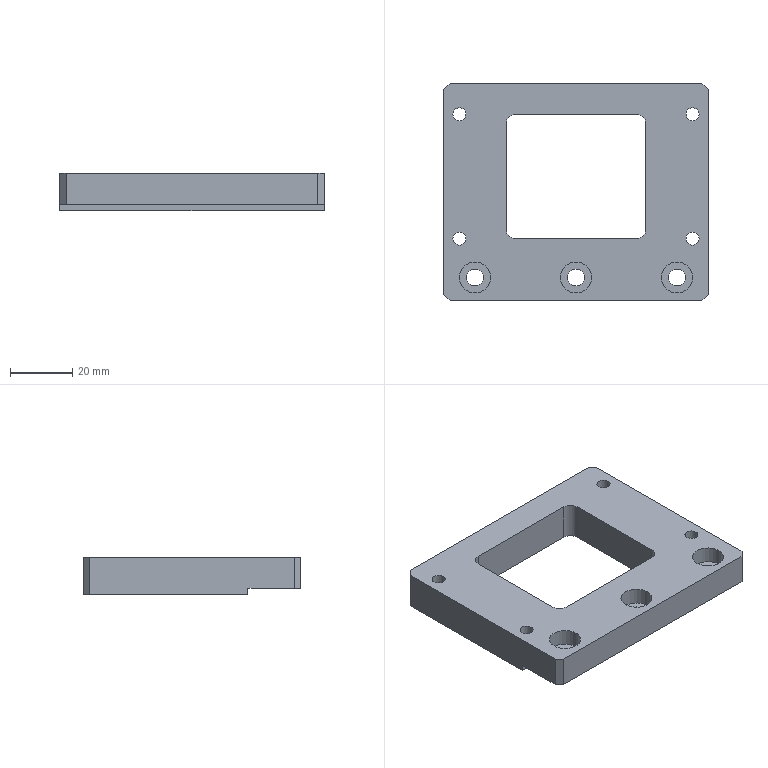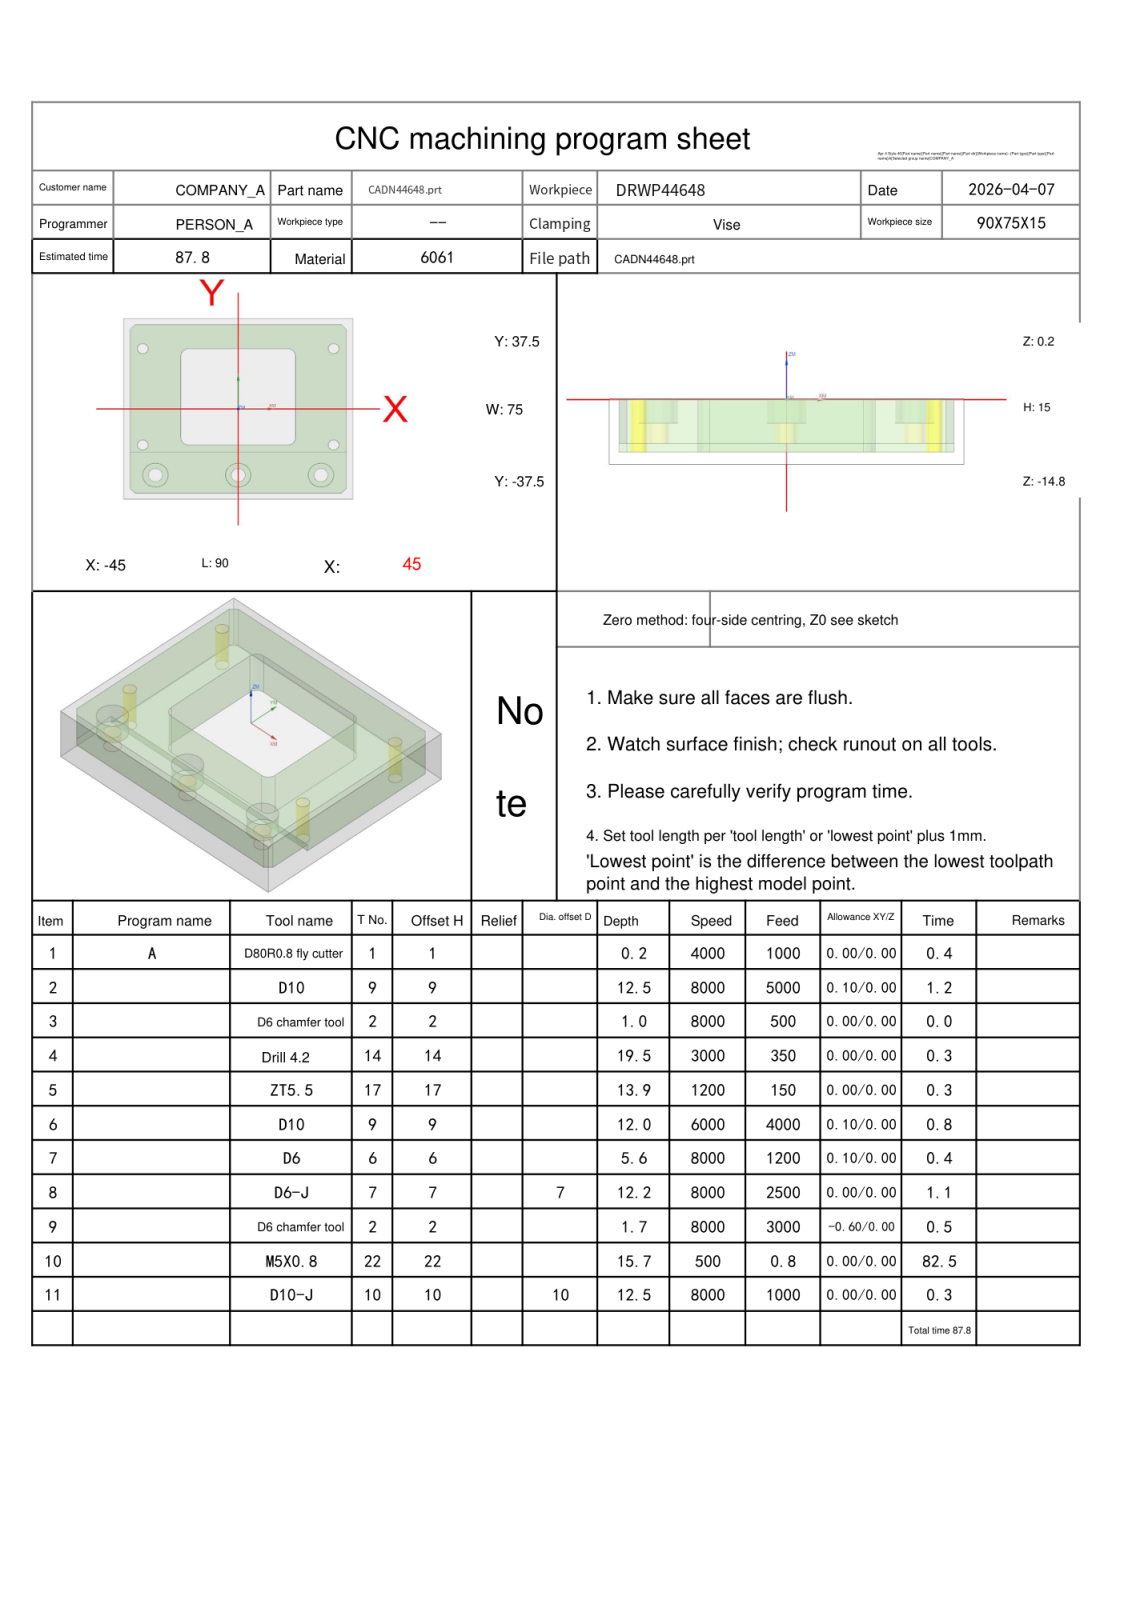NC program | NX | posted by the shop | part box 85 x 70 x 12 mm
Lines 1 to 579 of 5800:
%
O0001
(Machine time: 167.60 MIN)
(===Total Tool:9===)
(T1=D80R0.8 fly cutter D=80.  R=0.8  D-  H01 Z=0.    )
(T9=D10     D=10.  R=0.   D-  H09 Z=-12.3 )
(T2=D6 chamfer tool   D=6.   R=0.   D-  H02 Z=-1.5  )
(T14=drill 4.2  D=4.2  DR_a=118 D-  H14 Z=-19.26)
(T17=ZT5.5  D=5.5  DR_a=118 D-  H17 Z=-13.65)
(T6=D6      D=6.   R=0.   D-  H06 Z=-5.4  )
(T7=D6-J    D=6.   R=0.   D7  H07 Z=-12.  )
(T22=M5X0.8 D=4.2  DR_a=180 D-  H22 Z=-15.5 )
(T10=D10-J  D=10.  R=0.   D10 H10 Z=-12.3 )
G80 G90 G17 G49 G40
G91 G28 Z0
M01
N1 T01 M06
(D80R0.8 fly cutter  D=80. R=0.8 H=01 ce=0.00 di=0.00)
G00 G90 G54 X-87.5 Y25. M03 S4000
G43 H01 Z20.
M08
Z2.
G01 Z0.0 F1000.
X-82.5
X82.5
Y-25.
X-82.5
X-87.5
Z2.
G00 Z20.
G91 G28 Z0.0
M05
M09
G91 G28 Z0.0
M01
N2 T09 M06
(D10  D=10. R=0. H=09 ce=0.10 di=0.00)
G00 G90 G54 X0.0 Y40.1 M03 S8000
G43 H09 Z20.
M08
Z.5
G01 X40.5 Z.404 F5000.
G02 X44.106 Y38.606 Z.394 I0.0 J-5.1
G01 X46.106 Y36.606 Z.388
G02 X47.6 Y33. Z.378 I-3.606 J-3.606
G01 Y-33. Z.222
G02 X46.106 Y-36.606 Z.212 I-5.1 J0.0
G01 X44.106 Y-38.606 Z.206
G02 X40.5 Y-40.1 Z.196 I-3.606 J3.606
G01 X-40.5 Z.004
G02 X-44.106 Y-38.606 Z-.006 I0.0 J5.1
G01 X-46.106 Y-36.606 Z-.012
G02 X-47.6 Y-33. Z-.022 I3.606 J3.606
G01 Y33. Z-.178
G02 X-46.106 Y36.606 Z-.188 I5.1 J0.0
G01 X-44.106 Y38.606 Z-.194
G02 X-40.5 Y40.1 Z-.204 I3.606 J-3.606
G01 X40.5 Z-.396
G02 X44.106 Y38.606 Z-.406 I0.0 J-5.1
G01 X46.106 Y36.606 Z-.412
G02 X47.6 Y33. Z-.422 I-3.606 J-3.606
G01 Y-33. Z-.578
G02 X46.106 Y-36.606 Z-.588 I-5.1 J0.0
G01 X44.106 Y-38.606 Z-.594
G02 X40.5 Y-40.1 Z-.604 I-3.606 J3.606
G01 X-40.5 Z-.796
G02 X-44.106 Y-38.606 Z-.806 I0.0 J5.1
G01 X-46.106 Y-36.606 Z-.812
G02 X-47.6 Y-33. Z-.822 I3.606 J3.606
G01 Y33. Z-.978
G02 X-46.106 Y36.606 Z-.988 I5.1 J0.0
G01 X-44.106 Y38.606 Z-.994
G02 X-40.5 Y40.1 Z-1.004 I3.606 J-3.606
G01 X40.5 Z-1.196
G02 X44.106 Y38.606 Z-1.206 I0.0 J-5.1
G01 X46.106 Y36.606 Z-1.212
G02 X47.6 Y33. Z-1.222 I-3.606 J-3.606
G01 Y-33. Z-1.378
G02 X46.106 Y-36.606 Z-1.388 I-5.1 J0.0
G01 X44.106 Y-38.606 Z-1.394
G02 X40.5 Y-40.1 Z-1.404 I-3.606 J3.606
G01 X-40.5 Z-1.596
G02 X-44.106 Y-38.606 Z-1.606 I0.0 J5.1
G01 X-46.106 Y-36.606 Z-1.612
G02 X-47.6 Y-33. Z-1.622 I3.606 J3.606
G01 Y33. Z-1.778
G02 X-46.106 Y36.606 Z-1.788 I5.1 J0.0
G01 X-44.106 Y38.606 Z-1.794
G02 X-40.5 Y40.1 Z-1.804 I3.606 J-3.606
G01 X40.5 Z-1.996
G02 X44.106 Y38.606 Z-2.006 I0.0 J-5.1
G01 X46.106 Y36.606 Z-2.012
G02 X47.6 Y33. Z-2.022 I-3.606 J-3.606
G01 Y-33. Z-2.178
G02 X46.106 Y-36.606 Z-2.188 I-5.1 J0.0
G01 X44.106 Y-38.606 Z-2.194
G02 X40.5 Y-40.1 Z-2.204 I-3.606 J3.606
G01 X-40.5 Z-2.396
G02 X-44.106 Y-38.606 Z-2.406 I0.0 J5.1
G01 X-46.106 Y-36.606 Z-2.412
G02 X-47.6 Y-33. Z-2.422 I3.606 J3.606
G01 Y33. Z-2.578
G02 X-46.106 Y36.606 Z-2.588 I5.1 J0.0
G01 X-44.106 Y38.606 Z-2.594
G02 X-40.5 Y40.1 Z-2.604 I3.606 J-3.606
G01 X40.5 Z-2.796
G02 X44.106 Y38.606 Z-2.806 I0.0 J-5.1
G01 X46.106 Y36.606 Z-2.812
G02 X47.6 Y33. Z-2.822 I-3.606 J-3.606
G01 Y-33. Z-2.978
G02 X46.106 Y-36.606 Z-2.988 I-5.1 J0.0
G01 X44.106 Y-38.606 Z-2.994
G02 X40.5 Y-40.1 Z-3.004 I-3.606 J3.606
G01 X-40.5 Z-3.196
G02 X-44.106 Y-38.606 Z-3.206 I0.0 J5.1
G01 X-46.106 Y-36.606 Z-3.212
G02 X-47.6 Y-33. Z-3.222 I3.606 J3.606
G01 Y33. Z-3.378
G02 X-46.106 Y36.606 Z-3.388 I5.1 J0.0
G01 X-44.106 Y38.606 Z-3.394
G02 X-40.5 Y40.1 Z-3.404 I3.606 J-3.606
G01 X40.5 Z-3.596
G02 X44.106 Y38.606 Z-3.606 I0.0 J-5.1
G01 X46.106 Y36.606 Z-3.612
G02 X47.6 Y33. Z-3.622 I-3.606 J-3.606
G01 Y-33. Z-3.778
G02 X46.106 Y-36.606 Z-3.788 I-5.1 J0.0
G01 X44.106 Y-38.606 Z-3.794
G02 X40.5 Y-40.1 Z-3.804 I-3.606 J3.606
G01 X-40.5 Z-3.996
G02 X-44.106 Y-38.606 Z-4.006 I0.0 J5.1
G01 X-46.106 Y-36.606 Z-4.012
G02 X-47.6 Y-33. Z-4.022 I3.606 J3.606
G01 Y33. Z-4.178
G02 X-46.106 Y36.606 Z-4.188 I5.1 J0.0
G01 X-44.106 Y38.606 Z-4.194
G02 X-40.5 Y40.1 Z-4.204 I3.606 J-3.606
G01 X40.5 Z-4.396
G02 X44.106 Y38.606 Z-4.406 I0.0 J-5.1
G01 X46.106 Y36.606 Z-4.412
G02 X47.6 Y33. Z-4.422 I-3.606 J-3.606
G01 Y-33. Z-4.578
G02 X46.106 Y-36.606 Z-4.588 I-5.1 J0.0
G01 X44.106 Y-38.606 Z-4.594
G02 X40.5 Y-40.1 Z-4.604 I-3.606 J3.606
G01 X-40.5 Z-4.796
G02 X-44.106 Y-38.606 Z-4.806 I0.0 J5.1
G01 X-46.106 Y-36.606 Z-4.812
G02 X-47.6 Y-33. Z-4.822 I3.606 J3.606
G01 Y33. Z-4.978
G02 X-46.106 Y36.606 Z-4.988 I5.1 J0.0
G01 X-44.106 Y38.606 Z-4.994
G02 X-40.5 Y40.1 Z-5.004 I3.606 J-3.606
G01 X40.5 Z-5.196
G02 X44.106 Y38.606 Z-5.206 I0.0 J-5.1
G01 X46.106 Y36.606 Z-5.212
G02 X47.6 Y33. Z-5.222 I-3.606 J-3.606
G01 Y-33. Z-5.378
G02 X46.106 Y-36.606 Z-5.388 I-5.1 J0.0
G01 X44.106 Y-38.606 Z-5.394
G02 X40.5 Y-40.1 Z-5.404 I-3.606 J3.606
G01 X-40.5 Z-5.596
G02 X-44.106 Y-38.606 Z-5.606 I0.0 J5.1
G01 X-46.106 Y-36.606 Z-5.612
G02 X-47.6 Y-33. Z-5.622 I3.606 J3.606
G01 Y33. Z-5.778
G02 X-46.106 Y36.606 Z-5.788 I5.1 J0.0
G01 X-44.106 Y38.606 Z-5.794
G02 X-40.5 Y40.1 Z-5.804 I3.606 J-3.606
G01 X40.5 Z-5.996
G02 X44.106 Y38.606 Z-6.006 I0.0 J-5.1
G01 X46.106 Y36.606 Z-6.012
G02 X47.6 Y33. Z-6.022 I-3.606 J-3.606
G01 Y-33. Z-6.178
G02 X46.106 Y-36.606 Z-6.188 I-5.1 J0.0
G01 X44.106 Y-38.606 Z-6.194
G02 X40.5 Y-40.1 Z-6.204 I-3.606 J3.606
G01 X-40.5 Z-6.396
G02 X-44.106 Y-38.606 Z-6.406 I0.0 J5.1
G01 X-46.106 Y-36.606 Z-6.412
G02 X-47.6 Y-33. Z-6.422 I3.606 J3.606
G01 Y33. Z-6.578
G02 X-46.106 Y36.606 Z-6.588 I5.1 J0.0
G01 X-44.106 Y38.606 Z-6.594
G02 X-40.5 Y40.1 Z-6.604 I3.606 J-3.606
G01 X40.5 Z-6.796
G02 X44.106 Y38.606 Z-6.806 I0.0 J-5.1
G01 X46.106 Y36.606 Z-6.812
G02 X47.6 Y33. Z-6.822 I-3.606 J-3.606
G01 Y-33. Z-6.978
G02 X46.106 Y-36.606 Z-6.988 I-5.1 J0.0
G01 X44.106 Y-38.606 Z-6.994
G02 X40.5 Y-40.1 Z-7.004 I-3.606 J3.606
G01 X-40.5 Z-7.196
G02 X-44.106 Y-38.606 Z-7.206 I0.0 J5.1
G01 X-46.106 Y-36.606 Z-7.212
G02 X-47.6 Y-33. Z-7.222 I3.606 J3.606
G01 Y33. Z-7.378
G02 X-46.106 Y36.606 Z-7.388 I5.1 J0.0
G01 X-44.106 Y38.606 Z-7.394
G02 X-40.5 Y40.1 Z-7.404 I3.606 J-3.606
G01 X40.5 Z-7.596
G02 X44.106 Y38.606 Z-7.606 I0.0 J-5.1
G01 X46.106 Y36.606 Z-7.612
G02 X47.6 Y33. Z-7.622 I-3.606 J-3.606
G01 Y-33. Z-7.778
G02 X46.106 Y-36.606 Z-7.788 I-5.1 J0.0
G01 X44.106 Y-38.606 Z-7.794
G02 X40.5 Y-40.1 Z-7.804 I-3.606 J3.606
G01 X-40.5 Z-7.996
G02 X-44.106 Y-38.606 Z-8.006 I0.0 J5.1
G01 X-46.106 Y-36.606 Z-8.012
G02 X-47.6 Y-33. Z-8.022 I3.606 J3.606
G01 Y33. Z-8.178
G02 X-46.106 Y36.606 Z-8.188 I5.1 J0.0
G01 X-44.106 Y38.606 Z-8.194
G02 X-40.5 Y40.1 Z-8.204 I3.606 J-3.606
G01 X40.5 Z-8.396
G02 X44.106 Y38.606 Z-8.406 I0.0 J-5.1
G01 X46.106 Y36.606 Z-8.412
G02 X47.6 Y33. Z-8.422 I-3.606 J-3.606
G01 Y-33. Z-8.578
G02 X46.106 Y-36.606 Z-8.588 I-5.1 J0.0
G01 X44.106 Y-38.606 Z-8.594
G02 X40.5 Y-40.1 Z-8.604 I-3.606 J3.606
G01 X-40.5 Z-8.796
G02 X-44.106 Y-38.606 Z-8.806 I0.0 J5.1
G01 X-46.106 Y-36.606 Z-8.812
G02 X-47.6 Y-33. Z-8.822 I3.606 J3.606
G01 Y33. Z-8.978
G02 X-46.106 Y36.606 Z-8.988 I5.1 J0.0
G01 X-44.106 Y38.606 Z-8.994
G02 X-40.5 Y40.1 Z-9.004 I3.606 J-3.606
G01 X40.5 Z-9.196
G02 X44.106 Y38.606 Z-9.206 I0.0 J-5.1
G01 X46.106 Y36.606 Z-9.212
G02 X47.6 Y33. Z-9.222 I-3.606 J-3.606
G01 Y-33. Z-9.378
G02 X46.106 Y-36.606 Z-9.388 I-5.1 J0.0
G01 X44.106 Y-38.606 Z-9.394
G02 X40.5 Y-40.1 Z-9.404 I-3.606 J3.606
G01 X-40.5 Z-9.596
G02 X-44.106 Y-38.606 Z-9.606 I0.0 J5.1
G01 X-46.106 Y-36.606 Z-9.612
G02 X-47.6 Y-33. Z-9.622 I3.606 J3.606
G01 Y33. Z-9.778
G02 X-46.106 Y36.606 Z-9.788 I5.1 J0.0
G01 X-44.106 Y38.606 Z-9.794
G02 X-40.5 Y40.1 Z-9.804 I3.606 J-3.606
G01 X40.5 Z-9.996
G02 X44.106 Y38.606 Z-10.006 I0.0 J-5.1
G01 X46.106 Y36.606 Z-10.012
G02 X47.6 Y33. Z-10.022 I-3.606 J-3.606
G01 Y-33. Z-10.178
G02 X46.106 Y-36.606 Z-10.188 I-5.1 J0.0
G01 X44.106 Y-38.606 Z-10.194
G02 X40.5 Y-40.1 Z-10.204 I-3.606 J3.606
G01 X-40.5 Z-10.396
G02 X-44.106 Y-38.606 Z-10.406 I0.0 J5.1
G01 X-46.106 Y-36.606 Z-10.412
G02 X-47.6 Y-33. Z-10.422 I3.606 J3.606
G01 Y33. Z-10.578
G02 X-46.106 Y36.606 Z-10.588 I5.1 J0.0
G01 X-44.106 Y38.606 Z-10.594
G02 X-40.5 Y40.1 Z-10.604 I3.606 J-3.606
G01 X40.5 Z-10.796
G02 X44.106 Y38.606 Z-10.806 I0.0 J-5.1
G01 X46.106 Y36.606 Z-10.812
G02 X47.6 Y33. Z-10.822 I-3.606 J-3.606
G01 Y-33. Z-10.978
G02 X46.106 Y-36.606 Z-10.988 I-5.1 J0.0
G01 X44.106 Y-38.606 Z-10.994
G02 X40.5 Y-40.1 Z-11.004 I-3.606 J3.606
G01 X-40.5 Z-11.196
G02 X-44.106 Y-38.606 Z-11.206 I0.0 J5.1
G01 X-46.106 Y-36.606 Z-11.212
G02 X-47.6 Y-33. Z-11.222 I3.606 J3.606
G01 Y33. Z-11.378
G02 X-46.106 Y36.606 Z-11.388 I5.1 J0.0
G01 X-44.106 Y38.606 Z-11.394
G02 X-40.5 Y40.1 Z-11.404 I3.606 J-3.606
G01 X40.5 Z-11.596
G02 X44.106 Y38.606 Z-11.606 I0.0 J-5.1
G01 X46.106 Y36.606 Z-11.612
G02 X47.6 Y33. Z-11.622 I-3.606 J-3.606
G01 Y-33. Z-11.778
G02 X46.106 Y-36.606 Z-11.788 I-5.1 J0.0
G01 X44.106 Y-38.606 Z-11.794
G02 X40.5 Y-40.1 Z-11.804 I-3.606 J3.606
G01 X-40.5 Z-11.996
G02 X-44.106 Y-38.606 Z-12.006 I0.0 J5.1
G01 X-46.106 Y-36.606 Z-12.012
G02 X-47.6 Y-33. Z-12.022 I3.606 J3.606
G01 Y33. Z-12.178
G02 X-46.106 Y36.606 Z-12.188 I5.1 J0.0
G01 X-44.106 Y38.606 Z-12.194
G02 X-40.5 Y40.1 Z-12.204 I3.606 J-3.606
G01 X0.0 Z-12.3
X40.5
G02 X44.106 Y38.606 I0.0 J-5.1
G01 X46.106 Y36.606
G02 X47.6 Y33. I-3.606 J-3.606
G01 Y-33.
G02 X46.106 Y-36.606 I-5.1 J0.0
G01 X44.106 Y-38.606
G02 X40.5 Y-40.1 I-3.606 J3.606
G01 X-40.5
G02 X-44.106 Y-38.606 I0.0 J5.1
G01 X-46.106 Y-36.606
G02 X-47.6 Y-33. I3.606 J3.606
G01 Y33.
G02 X-46.106 Y36.606 I5.1 J0.0
G01 X-44.106 Y38.606
G02 X-40.5 Y40.1 I3.606 J-3.606
G01 X0.0
X.5
Z-11.3
G00 Z20.
G91 G28 Z0.0
M05
M09
G91 G28 Z0.0
M01
N3 T02 M06
(D6 chamfer tool  D=6. R=0. H=02 ce=0.00 di=0.00)
G00 G90 G54 X37.5 Y25. M03 S8000
G43 H02 Z20.
M08
G98 G81 X37.5 Y25. Z-.8 R1. F500.
Y-15.
X32.5 Y-27.5
X0.0
X-32.5
X-37.5 Y-15.
Y25.
G80
G00 Z20.
G91 G28 Z0.0
M05
M09
G91 G28 Z0.0
M01
N4 T14 M06
(drill 4.2 D=4.2 DR_a=118 H=14)
G00 G90 G54 X37.5 Y25. M03 S3000
G43 H14 Z20.
M08
G98 G83 X37.5 Y25. Z-19.262 R1. F350. Q3.
Y-15.
X-37.5
Y25.
G80
G00 Z20.
G91 G28 Z0.0
M05
M09
G91 G28 Z0.0
M01
N5 T17 M06
(ZT5.5 D=5.5 DR_a=118 H=17)
G00 G90 G54 X32.5 Y-27.5 M03 S1200
G43 H17 Z20.
M08
G98 G83 X32.5 Y-27.5 Z-13.652 R1. F150. Q2.
X0.0
X-32.5
G80
G00 Z20.
G91 G28 Z0.0
M05
M09
G91 G28 Z0.0
M01
N6 T09 M06
(D10  D=10. R=0. H=09 ce=0.10 di=0.00)
G00 G90 G54 X0.0 Y19.9 M03 S6000
G43 H09 Z20.
M08
Z.5
G01 X-17.4 Z.434 F4000.
Y-9.9 Z.32
X17.4 Z.188
Y19.9 Z.074
X-17.4 Z-.058
Y-9.9 Z-.172
X17.4 Z-.304
Y19.9 Z-.418
X-17.4 Z-.55
Y-9.9 Z-.664
X17.4 Z-.796
Y19.9 Z-.91
X-17.4 Z-1.042
Y-9.9 Z-1.156
X17.4 Z-1.288
Y19.9 Z-1.402
X-17.4 Z-1.534
Y-9.9 Z-1.648
X17.4 Z-1.78
Y19.9 Z-1.894
X-17.4 Z-2.026
Y-9.9 Z-2.14
X17.4 Z-2.272
Y19.9 Z-2.386
X-17.4 Z-2.518
Y-9.9 Z-2.632
X17.4 Z-2.764
Y19.9 Z-2.878
X-17.4 Z-3.01
Y-9.9 Z-3.124
X17.4 Z-3.256
Y19.9 Z-3.37
X-17.4 Z-3.502
Y-9.9 Z-3.616
X17.4 Z-3.748
Y19.9 Z-3.862
X-17.4 Z-3.994
Y-9.9 Z-4.108
X17.4 Z-4.24
Y19.9 Z-4.354
X-17.4 Z-4.486
Y-9.9 Z-4.6
X17.4 Z-4.732
Y19.9 Z-4.846
X-17.4 Z-4.978
Y-9.9 Z-5.092
X17.4 Z-5.224
Y19.9 Z-5.338
X-17.4 Z-5.47
Y-9.9 Z-5.584
X17.4 Z-5.716
Y19.9 Z-5.83
X-17.4 Z-5.962
Y-9.9 Z-6.076
X17.4 Z-6.208
Y19.9 Z-6.322
X-17.4 Z-6.454
Y-9.9 Z-6.568
X17.4 Z-6.7
Y19.9 Z-6.814
X-17.4 Z-6.946
Y-9.9 Z-7.06
X17.4 Z-7.192
Y19.9 Z-7.306
X-17.4 Z-7.438
Y-9.9 Z-7.552
X17.4 Z-7.684
Y19.9 Z-7.798
X-17.4 Z-7.93
Y-9.9 Z-8.044
X17.4 Z-8.176
Y19.9 Z-8.29
X-17.4 Z-8.422
Y-9.9 Z-8.536
X17.4 Z-8.668
Y19.9 Z-8.782
X-17.4 Z-8.914
Y-9.9 Z-9.028
X17.4 Z-9.16
Y19.9 Z-9.274
X-17.4 Z-9.406
Y-9.9 Z-9.52
X17.4 Z-9.652
Y19.9 Z-9.766
X-17.4 Z-9.898
Y-9.9 Z-10.012
X17.4 Z-10.144
Y19.9 Z-10.258
X-17.4 Z-10.39
Y-9.9 Z-10.504
X17.4 Z-10.636
Y19.9 Z-10.75
X-17.4 Z-10.882
Y-9.9 Z-10.996
X17.4 Z-11.128
Y19.9 Z-11.242
X-17.4 Z-11.374
Y-9.9 Z-11.488
X17.4 Z-11.62
Y19.9 Z-11.734
X0.0 Z-11.8
X-17.4
Y-9.9
X17.4
Y19.9
X0.0
X-.5
Z-10.8
G00 Z20.
G91 G28 Z0.0
M05
M09
G91 G28 Z0.0
M01
N7 T06 M06
(D6  D=6. R=0. H=06 ce=0.10 di=0.00)
G00 G90 G54 X32.5 Y-27.5 M03 S8000
G43 H06 Z20.
M08
Z.5
G03 X33.45 Y-28.45 I.95 J0.0 F1200.
X34.4 Y-27.5 I0.0 J.95
X34.4 Y-27.5 Z0.0 I-1.9 J0.0
X34.4 Y-27.5 Z-.5 I-1.9 J0.0
X34.4 Y-27.5 Z-1. I-1.9 J0.0
X34.4 Y-27.5 Z-1.5 I-1.9 J0.0
X34.4 Y-27.5 Z-2. I-1.9 J0.0
X34.4 Y-27.5 Z-2.5 I-1.9 J0.0
X34.4 Y-27.5 Z-3. I-1.9 J0.0
X34.4 Y-27.5 Z-3.5 I-1.9 J0.0
X34.4 Y-27.5 Z-4. I-1.9 J0.0
X34.4 Y-27.5 Z-4.5 I-1.9 J0.0
X34.4 Y-27.5 Z-5. I-1.9 J0.0
X33.087 Y-29.307 Z-5.4 I-1.9 J0.0
X34.4 Y-27.5 I-.587 J1.807
X32.5 Y-25.6 I-1.9 J0.0
X30.6 Y-27.5 I0.0 J-1.9
X32.5 Y-29.4 I1.9 J0.0
X33.087 Y-29.307 I0.0 J1.9
X33.744 Y-28.404 I-.294 J.904
X32.794 Y-27.454 I-.95 J0.0
X32.5 Y-27.5 I0.0 J-.95
G00 Z20.
X0.0
Z.5
G03 X.95 Y-28.45 I.95 J0.0
X1.9 Y-27.5 I0.0 J.95
X1.9 Y-27.5 Z0.0 I-1.9 J0.0
X1.9 Y-27.5 Z-.5 I-1.9 J0.0
X1.9 Y-27.5 Z-1. I-1.9 J0.0
X1.9 Y-27.5 Z-1.5 I-1.9 J0.0
X1.9 Y-27.5 Z-2. I-1.9 J0.0
X1.9 Y-27.5 Z-2.5 I-1.9 J0.0
X1.9 Y-27.5 Z-3. I-1.9 J0.0
X1.9 Y-27.5 Z-3.5 I-1.9 J0.0
X1.9 Y-27.5 Z-4. I-1.9 J0.0
X1.9 Y-27.5 Z-4.5 I-1.9 J0.0
X1.9 Y-27.5 Z-5. I-1.9 J0.0
X.587 Y-29.307 Z-5.4 I-1.9 J0.0
X1.9 Y-27.5 I-.587 J1.807
X0.0 Y-25.6 I-1.9 J0.0
X-1.9 Y-27.5 I0.0 J-1.9
X0.0 Y-29.4 I1.9 J0.0
X.587 Y-29.307 I0.0 J1.9
X1.244 Y-28.404 I-.294 J.904
X.294 Y-27.454 I-.95 J0.0
X0.0 Y-27.5 I0.0 J-.95
G00 Z20.
X-32.5
Z.5
G03 X-31.55 Y-28.45 I.95 J0.0
X-30.6 Y-27.5 I0.0 J.95
X-30.6 Y-27.5 Z0.0 I-1.9 J0.0
X-30.6 Y-27.5 Z-.5 I-1.9 J0.0
X-30.6 Y-27.5 Z-1. I-1.9 J0.0
X-30.6 Y-27.5 Z-1.5 I-1.9 J0.0
X-30.6 Y-27.5 Z-2. I-1.9 J0.0
X-30.6 Y-27.5 Z-2.5 I-1.9 J0.0
X-30.6 Y-27.5 Z-3. I-1.9 J0.0
X-30.6 Y-27.5 Z-3.5 I-1.9 J0.0
X-30.6 Y-27.5 Z-4. I-1.9 J0.0
X-30.6 Y-27.5 Z-4.5 I-1.9 J0.0
X-30.6 Y-27.5 Z-5. I-1.9 J0.0
X-31.913 Y-29.307 Z-5.4 I-1.9 J0.0
X-30.6 Y-27.5 I-.587 J1.807
X-32.5 Y-25.6 I-1.9 J0.0
X-34.4 Y-27.5 I0.0 J-1.9
X-32.5 Y-29.4 I1.9 J0.0
X-31.913 Y-29.307 I0.0 J1.9
X-31.256 Y-28.404 I-.294 J.904
X-32.206 Y-27.454 I-.95 J0.0
X-32.5 Y-27.5 I0.0 J-.95
G00 Z20.
G91 G28 Z0.0
M05
M09
G91 G28 Z0.0
M01